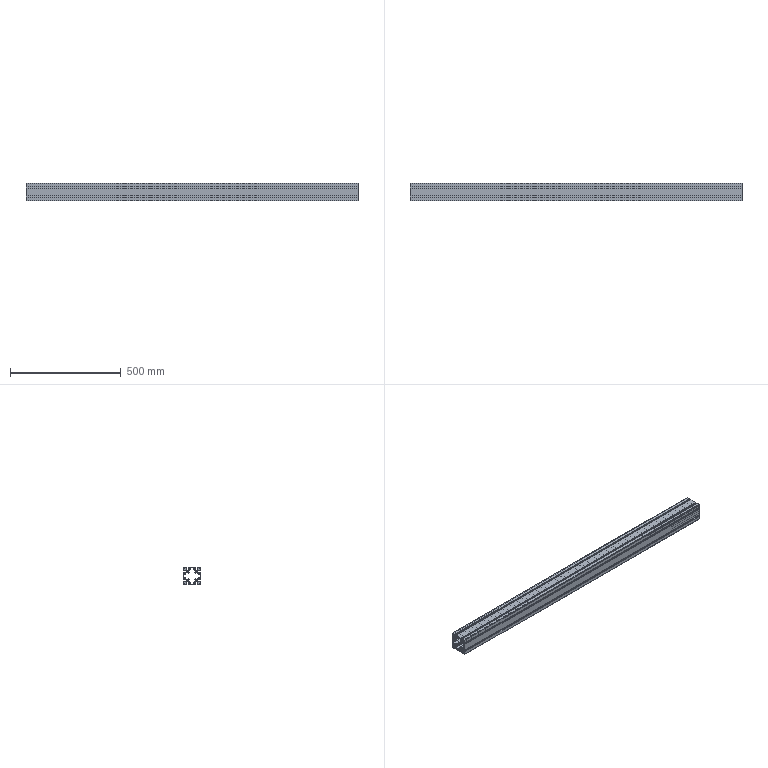Part | SolidWorks | features ICE 1, WeldMemberFeat 1, WeldmentFeature 1 | 1 solid | 174 faces | box 1500 x 80 x 80 mm | volume 3433531 mm3 | plane 146 | cylinder 28 | commonest cylinder face diameters 2 x8 6 x8 6.8 x8 3 x4